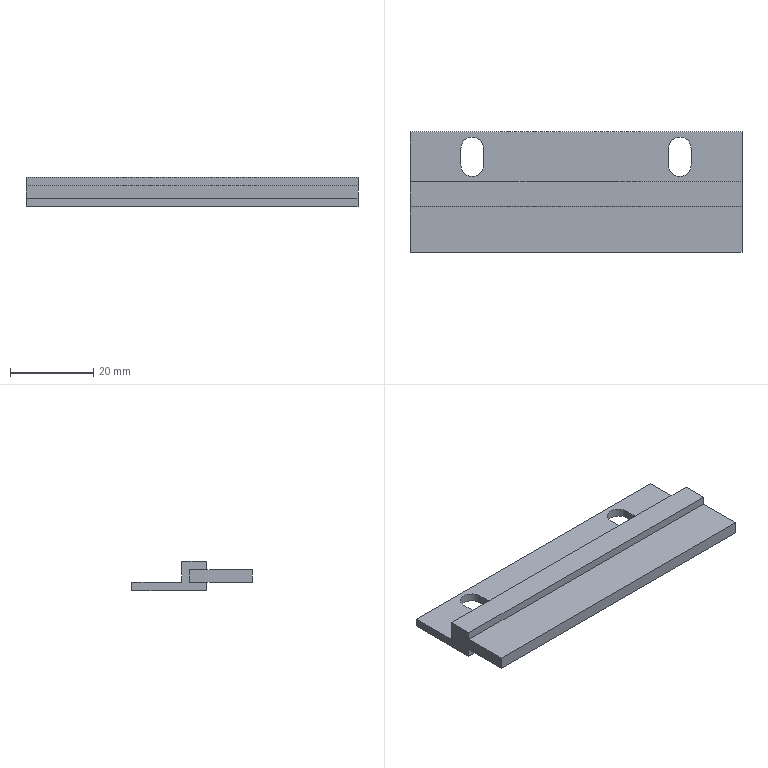Part | SolidWorks | features ICE 4, Extrusion 1, MirrorPattern 1 | 2 solids | 26 faces | box 80 x 29 x 7 mm | volume 7737 mm3 | plane 22 | cylinder 4 | commonest cylinder face diameters 5.5 x4
STEP:
#1=CARTESIAN_POINT('',(-40.,4.,5.));
#2=VERTEX_POINT('',#1);
#3=CARTESIAN_POINT('',(-40.,4.,2.));
#4=VERTEX_POINT('',#3);
#5=CARTESIAN_POINT('',(-40.,4.,5.));
#6=DIRECTION('',(0.,0.,-1.));
#7=VECTOR('',#6,1000.);
#8=LINE('',#5,#7);
#9=EDGE_CURVE('',#2,#4,#8,.T.);
#10=ORIENTED_EDGE('',*,*,#9,.T.);
#11=CARTESIAN_POINT('',(-40.,-11.,2.));
#12=VERTEX_POINT('',#11);
#13=CARTESIAN_POINT('',(-40.,-11.,2.));
#14=DIRECTION('',(0.,1.,0.));
#15=VECTOR('',#14,1000.);
#16=LINE('',#13,#15);
#17=EDGE_CURVE('',#12,#4,#16,.T.);
#18=ORIENTED_EDGE('',*,*,#17,.F.);
#19=CARTESIAN_POINT('',(-40.,-11.,5.));
#20=VERTEX_POINT('',#19);
#21=CARTESIAN_POINT('',(-40.,-11.,5.));
#22=DIRECTION('',(0.,0.,-1.));
#23=VECTOR('',#22,1000.);
#24=LINE('',#21,#23);
#25=EDGE_CURVE('',#20,#12,#24,.T.);
#26=ORIENTED_EDGE('',*,*,#25,.F.);
#27=CARTESIAN_POINT('',(-40.,-11.,5.));
#28=DIRECTION('',(0.,1.,0.));
#29=VECTOR('',#28,1000.);
#30=LINE('',#27,#29);
#31=EDGE_CURVE('',#20,#2,#30,.T.);
#32=ORIENTED_EDGE('',*,*,#31,.T.);
#33=EDGE_LOOP('',(#10,#18,#26,#32));
#34=FACE_OUTER_BOUND('',#33,.T.);
#35=CARTESIAN_POINT('',(-40.,-11.,5.));
#36=DIRECTION('',(1.,0.,0.));
#37=DIRECTION('',(0.,0.,-1.));
#38=AXIS2_PLACEMENT_3D('',#35,#36,#37);
#39=PLANE('',#38);
#40=ADVANCED_FACE('',(#34),#39,.F.);
#41=CARTESIAN_POINT('',(40.,4.,2.));
#42=VERTEX_POINT('',#41);
#43=CARTESIAN_POINT('',(-40.,4.,2.));
#44=DIRECTION('',(1.,0.,0.));
#45=VECTOR('',#44,1000.);
#46=LINE('',#43,#45);
#47=EDGE_CURVE('',#4,#42,#46,.T.);
#48=ORIENTED_EDGE('',*,*,#47,.T.);
#49=CARTESIAN_POINT('',(40.,-11.,2.));
#50=VERTEX_POINT('',#49);
#51=CARTESIAN_POINT('',(40.,-11.,2.));
#52=DIRECTION('',(0.,1.,0.));
#53=VECTOR('',#52,1000.);
#54=LINE('',#51,#53);
#55=EDGE_CURVE('',#50,#42,#54,.T.);
#56=ORIENTED_EDGE('',*,*,#55,.F.);
#57=CARTESIAN_POINT('',(-40.,-11.,2.));
#58=DIRECTION('',(1.,0.,0.));
#59=VECTOR('',#58,1000.);
#60=LINE('',#57,#59);
#61=EDGE_CURVE('',#12,#50,#60,.T.);
#62=ORIENTED_EDGE('',*,*,#61,.F.);
#63=ORIENTED_EDGE('',*,*,#17,.T.);
#64=EDGE_LOOP('',(#48,#56,#62,#63));
#65=FACE_OUTER_BOUND('',#64,.T.);
#66=CARTESIAN_POINT('',(-40.,-11.,2.));
#67=DIRECTION('',(0.,0.,1.));
#68=DIRECTION('',(1.,0.,0.));
#69=AXIS2_PLACEMENT_3D('',#66,#67,#68);
#70=PLANE('',#69);
#71=ADVANCED_FACE('',(#65),#70,.F.);
#72=CARTESIAN_POINT('',(40.,4.,5.));
#73=VERTEX_POINT('',#72);
#74=CARTESIAN_POINT('',(40.,4.,2.));
#75=DIRECTION('',(0.,0.,1.));
#76=VECTOR('',#75,1000.);
#77=LINE('',#74,#76);
#78=EDGE_CURVE('',#42,#73,#77,.T.);
#79=ORIENTED_EDGE('',*,*,#78,.T.);
#80=CARTESIAN_POINT('',(40.,-11.,5.));
#81=VERTEX_POINT('',#80);
#82=CARTESIAN_POINT('',(40.,-11.,5.));
#83=DIRECTION('',(0.,1.,0.));
#84=VECTOR('',#83,1000.);
#85=LINE('',#82,#84);
#86=EDGE_CURVE('',#81,#73,#85,.T.);
#87=ORIENTED_EDGE('',*,*,#86,.F.);
#88=CARTESIAN_POINT('',(40.,-11.,2.));
#89=DIRECTION('',(0.,0.,1.));
#90=VECTOR('',#89,1000.);
#91=LINE('',#88,#90);
#92=EDGE_CURVE('',#50,#81,#91,.T.);
#93=ORIENTED_EDGE('',*,*,#92,.F.);
#94=ORIENTED_EDGE('',*,*,#55,.T.);
#95=EDGE_LOOP('',(#79,#87,#93,#94));
#96=FACE_OUTER_BOUND('',#95,.T.);
#97=CARTESIAN_POINT('',(40.,-11.,2.));
#98=DIRECTION('',(-1.,0.,0.));
#99=DIRECTION('',(0.,0.,1.));
#100=AXIS2_PLACEMENT_3D('',#97,#98,#99);
#101=PLANE('',#100);
#102=ADVANCED_FACE('',(#96),#101,.F.);
#103=CARTESIAN_POINT('',(40.,4.,5.));
#104=DIRECTION('',(-1.,0.,0.));
#105=VECTOR('',#104,1000.);
#106=LINE('',#103,#105);
#107=EDGE_CURVE('',#73,#2,#106,.T.);
#108=ORIENTED_EDGE('',*,*,#107,.T.);
#109=ORIENTED_EDGE('',*,*,#31,.F.);
#110=CARTESIAN_POINT('',(40.,-11.,5.));
#111=DIRECTION('',(-1.,0.,0.));
#112=VECTOR('',#111,1000.);
#113=LINE('',#110,#112);
#114=EDGE_CURVE('',#81,#20,#113,.T.);
#115=ORIENTED_EDGE('',*,*,#114,.F.);
#116=ORIENTED_EDGE('',*,*,#86,.T.);
#117=EDGE_LOOP('',(#108,#109,#115,#116));
#118=FACE_OUTER_BOUND('',#117,.T.);
#119=CARTESIAN_POINT('',(40.,-11.,5.));
#120=DIRECTION('',(0.,0.,-1.));
#121=DIRECTION('',(-1.,0.,0.));
#122=AXIS2_PLACEMENT_3D('',#119,#120,#121);
#123=PLANE('',#122);
#124=ADVANCED_FACE('',(#118),#123,.F.);
#125=ORIENTED_EDGE('',*,*,#25,.T.);
#126=ORIENTED_EDGE('',*,*,#61,.T.);
#127=ORIENTED_EDGE('',*,*,#92,.T.);
#128=ORIENTED_EDGE('',*,*,#114,.T.);
#129=EDGE_LOOP('',(#125,#126,#127,#128));
#130=FACE_OUTER_BOUND('',#129,.T.);
#131=CARTESIAN_POINT('',(0.,-11.,0.));
#132=DIRECTION('',(0.,-1.,0.));
#133=DIRECTION('',(0.,0.,-1.));
#134=AXIS2_PLACEMENT_3D('',#131,#132,#133);
#135=PLANE('',#134);
#136=ADVANCED_FACE('',(#130),#135,.T.);
#137=ORIENTED_EDGE('',*,*,#9,.F.);
#138=ORIENTED_EDGE('',*,*,#107,.F.);
#139=ORIENTED_EDGE('',*,*,#78,.F.);
#140=ORIENTED_EDGE('',*,*,#47,.F.);
#141=EDGE_LOOP('',(#137,#138,#139,#140));
#142=FACE_OUTER_BOUND('',#141,.T.);
#143=CARTESIAN_POINT('',(0.,4.,0.));
#144=DIRECTION('',(0.,-1.,0.));
#145=DIRECTION('',(0.,0.,-1.));
#146=AXIS2_PLACEMENT_3D('',#143,#144,#145);
#147=PLANE('',#146);
#148=ADVANCED_FACE('',(#142),#147,.F.);
#149=CLOSED_SHELL('',(#40,#71,#102,#124,#136,#148));
#150=MANIFOLD_SOLID_BREP('',#149);
#151=CARTESIAN_POINT('',(40.,6.,2.));
#152=VERTEX_POINT('',#151);
#153=CARTESIAN_POINT('',(-40.,6.,2.));
#154=VERTEX_POINT('',#153);
#155=CARTESIAN_POINT('',(-40.,6.,2.));
#156=DIRECTION('',(-1.,0.,0.));
#157=VECTOR('',#156,1000.);
#158=LINE('',#155,#157);
#159=EDGE_CURVE('',#152,#154,#158,.T.);
#160=ORIENTED_EDGE('',*,*,#159,.F.);
#161=CARTESIAN_POINT('',(40.,18.,2.));
#162=VERTEX_POINT('',#161);
#163=CARTESIAN_POINT('',(40.,18.,2.));
#164=DIRECTION('',(0.,1.,0.));
#165=VECTOR('',#164,1000.);
#166=LINE('',#163,#165);
#167=EDGE_CURVE('',#152,#162,#166,.T.);
#168=ORIENTED_EDGE('',*,*,#167,.T.);
#169=CARTESIAN_POINT('',(-40.,18.,2.));
#170=VERTEX_POINT('',#169);
#171=CARTESIAN_POINT('',(-40.,18.,2.));
#172=DIRECTION('',(-1.,0.,0.));
#173=VECTOR('',#172,1000.);
#174=LINE('',#171,#173);
#175=EDGE_CURVE('',#162,#170,#174,.T.);
#176=ORIENTED_EDGE('',*,*,#175,.T.);
#177=CARTESIAN_POINT('',(-40.,18.,2.));
#178=DIRECTION('',(0.,-1.,0.));
#179=VECTOR('',#178,1000.);
#180=LINE('',#177,#179);
#181=EDGE_CURVE('',#170,#154,#180,.T.);
#182=ORIENTED_EDGE('',*,*,#181,.T.);
#183=EDGE_LOOP('',(#160,#168,#176,#182));
#184=FACE_OUTER_BOUND('',#183,.T.);
#185=CARTESIAN_POINT('',(-22.25,14.,2.));
#186=VERTEX_POINT('',#185);
#187=CARTESIAN_POINT('',(-27.75,14.,2.));
#188=VERTEX_POINT('',#187);
#189=CARTESIAN_POINT('',(-25.,14.,2.));
#190=DIRECTION('',(0.,0.,1.));
#191=DIRECTION('',(1.,0.,0.));
#192=AXIS2_PLACEMENT_3D('',#189,#190,#191);
#193=CIRCLE('',#192,2.75);
#194=EDGE_CURVE('',#186,#188,#193,.T.);
#195=ORIENTED_EDGE('',*,*,#194,.F.);
#196=CARTESIAN_POINT('',(-22.25,10.,2.));
#197=VERTEX_POINT('',#196);
#198=CARTESIAN_POINT('',(-22.25,14.,2.));
#199=DIRECTION('',(0.,1.,0.));
#200=VECTOR('',#199,1000.);
#201=LINE('',#198,#200);
#202=EDGE_CURVE('',#197,#186,#201,.T.);
#203=ORIENTED_EDGE('',*,*,#202,.F.);
#204=CARTESIAN_POINT('',(-27.75,10.,2.));
#205=VERTEX_POINT('',#204);
#206=CARTESIAN_POINT('',(-25.,10.,2.));
#207=DIRECTION('',(0.,0.,1.));
#208=DIRECTION('',(1.,0.,0.));
#209=AXIS2_PLACEMENT_3D('',#206,#207,#208);
#210=CIRCLE('',#209,2.75);
#211=EDGE_CURVE('',#205,#197,#210,.T.);
#212=ORIENTED_EDGE('',*,*,#211,.F.);
#213=CARTESIAN_POINT('',(-27.75,14.,2.));
#214=DIRECTION('',(0.,-1.,0.));
#215=VECTOR('',#214,1000.);
#216=LINE('',#213,#215);
#217=EDGE_CURVE('',#188,#205,#216,.T.);
#218=ORIENTED_EDGE('',*,*,#217,.F.);
#219=EDGE_LOOP('',(#195,#203,#212,#218));
#220=FACE_BOUND('',#219,.T.);
#221=CARTESIAN_POINT('',(22.25,10.,2.));
#222=VERTEX_POINT('',#221);
#223=CARTESIAN_POINT('',(22.25,14.,2.));
#224=VERTEX_POINT('',#223);
#225=CARTESIAN_POINT('',(22.25,14.,2.));
#226=DIRECTION('',(0.,1.,0.));
#227=VECTOR('',#226,1000.);
#228=LINE('',#225,#227);
#229=EDGE_CURVE('',#222,#224,#228,.T.);
#230=ORIENTED_EDGE('',*,*,#229,.T.);
#231=CARTESIAN_POINT('',(27.75,14.,2.));
#232=VERTEX_POINT('',#231);
#233=CARTESIAN_POINT('',(25.,14.,2.));
#234=DIRECTION('',(0.,0.,-1.));
#235=DIRECTION('',(-1.,0.,0.));
#236=AXIS2_PLACEMENT_3D('',#233,#234,#235);
#237=CIRCLE('',#236,2.75);
#238=EDGE_CURVE('',#224,#232,#237,.T.);
#239=ORIENTED_EDGE('',*,*,#238,.T.);
#240=CARTESIAN_POINT('',(27.75,10.,2.));
#241=VERTEX_POINT('',#240);
#242=CARTESIAN_POINT('',(27.75,14.,2.));
#243=DIRECTION('',(0.,-1.,0.));
#244=VECTOR('',#243,1000.);
#245=LINE('',#242,#244);
#246=EDGE_CURVE('',#232,#241,#245,.T.);
#247=ORIENTED_EDGE('',*,*,#246,.T.);
#248=CARTESIAN_POINT('',(25.,10.,2.));
#249=DIRECTION('',(0.,0.,-1.));
#250=DIRECTION('',(-1.,0.,0.));
#251=AXIS2_PLACEMENT_3D('',#248,#249,#250);
#252=CIRCLE('',#251,2.75);
#253=EDGE_CURVE('',#241,#222,#252,.T.);
#254=ORIENTED_EDGE('',*,*,#253,.T.);
#255=EDGE_LOOP('',(#230,#239,#247,#254));
#256=FACE_BOUND('',#255,.T.);
#257=CARTESIAN_POINT('',(0.,0.,2.));
#258=DIRECTION('',(0.,0.,1.));
#259=DIRECTION('',(1.,0.,0.));
#260=AXIS2_PLACEMENT_3D('',#257,#258,#259);
#261=PLANE('',#260);
#262=ADVANCED_FACE('',(#184,#220,#256),#261,.T.);
#263=CARTESIAN_POINT('',(-40.,18.,0.));
#264=VERTEX_POINT('',#263);
#265=CARTESIAN_POINT('',(-40.,0.,0.));
#266=VERTEX_POINT('',#265);
#267=CARTESIAN_POINT('',(-40.,18.,0.));
#268=DIRECTION('',(0.,-1.,0.));
#269=VECTOR('',#268,1000.);
#270=LINE('',#267,#269);
#271=EDGE_CURVE('',#264,#266,#270,.T.);
#272=ORIENTED_EDGE('',*,*,#271,.F.);
#273=CARTESIAN_POINT('',(40.,18.,0.));
#274=VERTEX_POINT('',#273);
#275=CARTESIAN_POINT('',(-40.,18.,0.));
#276=DIRECTION('',(-1.,0.,0.));
#277=VECTOR('',#276,1000.);
#278=LINE('',#275,#277);
#279=EDGE_CURVE('',#274,#264,#278,.T.);
#280=ORIENTED_EDGE('',*,*,#279,.F.);
#281=CARTESIAN_POINT('',(40.,0.,0.));
#282=VERTEX_POINT('',#281);
#283=CARTESIAN_POINT('',(40.,18.,0.));
#284=DIRECTION('',(0.,1.,0.));
#285=VECTOR('',#284,1000.);
#286=LINE('',#283,#285);
#287=EDGE_CURVE('',#282,#274,#286,.T.);
#288=ORIENTED_EDGE('',*,*,#287,.F.);
#289=CARTESIAN_POINT('',(-40.,0.,0.));
#290=DIRECTION('',(1.,0.,0.));
#291=VECTOR('',#290,1000.);
#292=LINE('',#289,#291);
#293=EDGE_CURVE('',#266,#282,#292,.T.);
#294=ORIENTED_EDGE('',*,*,#293,.F.);
#295=EDGE_LOOP('',(#272,#280,#288,#294));
#296=FACE_OUTER_BOUND('',#295,.T.);
#297=CARTESIAN_POINT('',(-22.25,10.,0.));
#298=VERTEX_POINT('',#297);
#299=CARTESIAN_POINT('',(-22.25,14.,0.));
#300=VERTEX_POINT('',#299);
#301=CARTESIAN_POINT('',(-22.25,0.,0.));
#302=DIRECTION('',(0.,1.,0.));
#303=VECTOR('',#302,1000.);
#304=LINE('',#301,#303);
#305=EDGE_CURVE('',#298,#300,#304,.T.);
#306=ORIENTED_EDGE('',*,*,#305,.T.);
#307=CARTESIAN_POINT('',(-27.75,14.,0.));
#308=VERTEX_POINT('',#307);
#309=CARTESIAN_POINT('',(-25.,14.,0.));
#310=DIRECTION('',(0.,0.,1.));
#311=DIRECTION('',(1.,0.,0.));
#312=AXIS2_PLACEMENT_3D('',#309,#310,#311);
#313=CIRCLE('',#312,2.75);
#314=EDGE_CURVE('',#300,#308,#313,.T.);
#315=ORIENTED_EDGE('',*,*,#314,.T.);
#316=CARTESIAN_POINT('',(-27.75,10.,0.));
#317=VERTEX_POINT('',#316);
#318=CARTESIAN_POINT('',(-27.75,0.,0.));
#319=DIRECTION('',(0.,-1.,0.));
#320=VECTOR('',#319,1000.);
#321=LINE('',#318,#320);
#322=EDGE_CURVE('',#308,#317,#321,.T.);
#323=ORIENTED_EDGE('',*,*,#322,.T.);
#324=CARTESIAN_POINT('',(-25.,10.,0.));
#325=DIRECTION('',(0.,0.,1.));
#326=DIRECTION('',(1.,0.,0.));
#327=AXIS2_PLACEMENT_3D('',#324,#325,#326);
#328=CIRCLE('',#327,2.75);
#329=EDGE_CURVE('',#317,#298,#328,.T.);
#330=ORIENTED_EDGE('',*,*,#329,.T.);
#331=EDGE_LOOP('',(#306,#315,#323,#330));
#332=FACE_BOUND('',#331,.T.);
#333=CARTESIAN_POINT('',(22.25,14.,0.));
#334=VERTEX_POINT('',#333);
#335=CARTESIAN_POINT('',(27.75,14.,0.));
#336=VERTEX_POINT('',#335);
#337=CARTESIAN_POINT('',(25.,14.,0.));
#338=DIRECTION('',(0.,0.,-1.));
#339=DIRECTION('',(1.,0.,0.));
#340=AXIS2_PLACEMENT_3D('',#337,#338,#339);
#341=CIRCLE('',#340,2.75);
#342=EDGE_CURVE('',#334,#336,#341,.T.);
#343=ORIENTED_EDGE('',*,*,#342,.F.);
#344=CARTESIAN_POINT('',(22.25,10.,0.));
#345=VERTEX_POINT('',#344);
#346=CARTESIAN_POINT('',(22.25,0.,0.));
#347=DIRECTION('',(0.,1.,0.));
#348=VECTOR('',#347,1000.);
#349=LINE('',#346,#348);
#350=EDGE_CURVE('',#345,#334,#349,.T.);
#351=ORIENTED_EDGE('',*,*,#350,.F.);
#352=CARTESIAN_POINT('',(27.75,10.,0.));
#353=VERTEX_POINT('',#352);
#354=CARTESIAN_POINT('',(25.,10.,0.));
#355=DIRECTION('',(0.,0.,-1.));
#356=DIRECTION('',(1.,0.,0.));
#357=AXIS2_PLACEMENT_3D('',#354,#355,#356);
#358=CIRCLE('',#357,2.75);
#359=EDGE_CURVE('',#353,#345,#358,.T.);
#360=ORIENTED_EDGE('',*,*,#359,.F.);
#361=CARTESIAN_POINT('',(27.75,0.,0.));
#362=DIRECTION('',(0.,-1.,0.));
#363=VECTOR('',#362,1000.);
#364=LINE('',#361,#363);
#365=EDGE_CURVE('',#336,#353,#364,.T.);
#366=ORIENTED_EDGE('',*,*,#365,.F.);
#367=EDGE_LOOP('',(#343,#351,#360,#366));
#368=FACE_BOUND('',#367,.T.);
#369=CARTESIAN_POINT('',(0.,0.,0.));
#370=DIRECTION('',(0.,0.,1.));
#371=DIRECTION('',(1.,0.,0.));
#372=AXIS2_PLACEMENT_3D('',#369,#370,#371);
#373=PLANE('',#372);
#374=ADVANCED_FACE('',(#296,#332,#368),#373,.F.);
#375=ORIENTED_EDGE('',*,*,#271,.T.);
#376=CARTESIAN_POINT('',(-40.,0.,2.));
#377=VERTEX_POINT('',#376);
#378=CARTESIAN_POINT('',(-40.,0.,2.));
#379=DIRECTION('',(0.,0.,-1.));
#380=VECTOR('',#379,1000.);
#381=LINE('',#378,#380);
#382=EDGE_CURVE('',#377,#266,#381,.T.);
#383=ORIENTED_EDGE('',*,*,#382,.F.);
#384=CARTESIAN_POINT('',(-40.,4.,2.));
#385=VERTEX_POINT('',#384);
#386=CARTESIAN_POINT('',(-40.,18.,2.));
#387=DIRECTION('',(0.,-1.,0.));
#388=VECTOR('',#387,1000.);
#389=LINE('',#386,#388);
#390=EDGE_CURVE('',#385,#377,#389,.T.);
#391=ORIENTED_EDGE('',*,*,#390,.F.);
#392=CARTESIAN_POINT('',(-40.,4.,5.));
#393=VERTEX_POINT('',#392);
#394=CARTESIAN_POINT('',(-40.,4.,5.));
#395=DIRECTION('',(0.,0.,-1.));
#396=VECTOR('',#395,1000.);
#397=LINE('',#394,#396);
#398=EDGE_CURVE('',#393,#385,#397,.T.);
#399=ORIENTED_EDGE('',*,*,#398,.F.);
#400=CARTESIAN_POINT('',(-40.,0.,5.));
#401=VERTEX_POINT('',#400);
#402=CARTESIAN_POINT('',(-40.,-80.025,5.));
#403=DIRECTION('',(0.,1.,0.));
#404=VECTOR('',#403,1000.);
#405=LINE('',#402,#404);
#406=EDGE_CURVE('',#401,#393,#405,.T.);
#407=ORIENTED_EDGE('',*,*,#406,.F.);
#408=CARTESIAN_POINT('',(-40.,0.,7.));
#409=VERTEX_POINT('',#408);
#410=CARTESIAN_POINT('',(-40.,0.,5.));
#411=DIRECTION('',(0.,0.,-1.));
#412=VECTOR('',#411,1000.);
#413=LINE('',#410,#412);
#414=EDGE_CURVE('',#409,#401,#413,.T.);
#415=ORIENTED_EDGE('',*,*,#414,.F.);
#416=CARTESIAN_POINT('',(-40.,6.,7.));
#417=VERTEX_POINT('',#416);
#418=CARTESIAN_POINT('',(-40.,-80.025,7.));
#419=DIRECTION('',(0.,1.,0.));
#420=VECTOR('',#419,1000.);
#421=LINE('',#418,#420);
#422=EDGE_CURVE('',#409,#417,#421,.T.);
#423=ORIENTED_EDGE('',*,*,#422,.T.);
#424=CARTESIAN_POINT('',(-40.,6.,5.));
#425=DIRECTION('',(0.,0.,-1.));
#426=VECTOR('',#425,1000.);
#427=LINE('',#424,#426);
#428=EDGE_CURVE('',#417,#154,#427,.T.);
#429=ORIENTED_EDGE('',*,*,#428,.T.);
#430=ORIENTED_EDGE('',*,*,#181,.F.);
#431=CARTESIAN_POINT('',(-40.,18.,2.));
#432=DIRECTION('',(0.,0.,-1.));
#433=VECTOR('',#432,1000.);
#434=LINE('',#431,#433);
#435=EDGE_CURVE('',#170,#264,#434,.T.);
#436=ORIENTED_EDGE('',*,*,#435,.T.);
#437=EDGE_LOOP('',(#375,#383,#391,#399,#407,#415,#423,#429,#430,#436));
#438=FACE_OUTER_BOUND('',#437,.T.);
#439=CARTESIAN_POINT('',(-40.,18.,2.));
#440=DIRECTION('',(1.,0.,0.));
#441=DIRECTION('',(0.,1.,0.));
#442=AXIS2_PLACEMENT_3D('',#439,#440,#441);
#443=PLANE('',#442);
#444=ADVANCED_FACE('',(#438),#443,.F.);
#445=ORIENTED_EDGE('',*,*,#293,.T.);
#446=CARTESIAN_POINT('',(40.,0.,2.));
#447=VERTEX_POINT('',#446);
#448=CARTESIAN_POINT('',(40.,0.,2.));
#449=DIRECTION('',(0.,0.,-1.));
#450=VECTOR('',#449,1000.);
#451=LINE('',#448,#450);
#452=EDGE_CURVE('',#447,#282,#451,.T.);
#453=ORIENTED_EDGE('',*,*,#452,.F.);
#454=CARTESIAN_POINT('',(-40.,0.,2.));
#455=DIRECTION('',(1.,0.,0.));
#456=VECTOR('',#455,1000.);
#457=LINE('',#454,#456);
#458=EDGE_CURVE('',#377,#447,#457,.T.);
#459=ORIENTED_EDGE('',*,*,#458,.F.);
#460=ORIENTED_EDGE('',*,*,#382,.T.);
#461=EDGE_LOOP('',(#445,#453,#459,#460));
#462=FACE_OUTER_BOUND('',#461,.T.);
#463=CARTESIAN_POINT('',(-40.,0.,2.));
#464=DIRECTION('',(0.,1.,0.));
#465=DIRECTION('',(0.,0.,1.));
#466=AXIS2_PLACEMENT_3D('',#463,#464,#465);
#467=PLANE('',#466);
#468=ADVANCED_FACE('',(#462),#467,.F.);
#469=ORIENTED_EDGE('',*,*,#287,.T.);
#470=CARTESIAN_POINT('',(40.,18.,2.));
#471=DIRECTION('',(0.,0.,-1.));
#472=VECTOR('',#471,1000.);
#473=LINE('',#470,#472);
#474=EDGE_CURVE('',#162,#274,#473,.T.);
#475=ORIENTED_EDGE('',*,*,#474,.F.);
#476=ORIENTED_EDGE('',*,*,#167,.F.);
#477=CARTESIAN_POINT('',(40.,6.,7.));
#478=VERTEX_POINT('',#477);
#479=CARTESIAN_POINT('',(40.,6.,5.));
#480=DIRECTION('',(0.,0.,-1.));
#481=VECTOR('',#480,1000.);
#482=LINE('',#479,#481);
#483=EDGE_CURVE('',#478,#152,#482,.T.);
#484=ORIENTED_EDGE('',*,*,#483,.F.);
#485=CARTESIAN_POINT('',(40.,0.,7.));
#486=VERTEX_POINT('',#485);
#487=CARTESIAN_POINT('',(40.,-80.025,7.));
#488=DIRECTION('',(0.,1.,0.));
#489=VECTOR('',#488,1000.);
#490=LINE('',#487,#489);
#491=EDGE_CURVE('',#486,#478,#490,.T.);
#492=ORIENTED_EDGE('',*,*,#491,.F.);
#493=CARTESIAN_POINT('',(40.,0.,5.));
#494=VERTEX_POINT('',#493);
#495=CARTESIAN_POINT('',(40.,0.,5.));
#496=DIRECTION('',(0.,0.,1.));
#497=VECTOR('',#496,1000.);
#498=LINE('',#495,#497);
#499=EDGE_CURVE('',#494,#486,#498,.T.);
#500=ORIENTED_EDGE('',*,*,#499,.F.);
#501=CARTESIAN_POINT('',(40.,4.,5.));
#502=VERTEX_POINT('',#501);
#503=CARTESIAN_POINT('',(40.,-80.025,5.));
#504=DIRECTION('',(0.,1.,0.));
#505=VECTOR('',#504,1000.);
#506=LINE('',#503,#505);
#507=EDGE_CURVE('',#494,#502,#506,.T.);
#508=ORIENTED_EDGE('',*,*,#507,.T.);
#509=CARTESIAN_POINT('',(40.,4.,2.));
#510=VERTEX_POINT('',#509);
#511=CARTESIAN_POINT('',(40.,4.,5.));
#512=DIRECTION('',(0.,0.,-1.));
#513=VECTOR('',#512,1000.);
#514=LINE('',#511,#513);
#515=EDGE_CURVE('',#502,#510,#514,.T.);
#516=ORIENTED_EDGE('',*,*,#515,.T.);
#517=CARTESIAN_POINT('',(40.,18.,2.));
#518=DIRECTION('',(0.,1.,0.));
#519=VECTOR('',#518,1000.);
#520=LINE('',#517,#519);
#521=EDGE_CURVE('',#447,#510,#520,.T.);
#522=ORIENTED_EDGE('',*,*,#521,.F.);
#523=ORIENTED_EDGE('',*,*,#452,.T.);
#524=EDGE_LOOP('',(#469,#475,#476,#484,#492,#500,#508,#516,#522,#523));
#525=FACE_OUTER_BOUND('',#524,.T.);
#526=CARTESIAN_POINT('',(40.,18.,2.));
#527=DIRECTION('',(-1.,0.,0.));
#528=DIRECTION('',(0.,0.,1.));
#529=AXIS2_PLACEMENT_3D('',#526,#527,#528);
#530=PLANE('',#529);
#531=ADVANCED_FACE('',(#525),#530,.F.);
#532=ORIENTED_EDGE('',*,*,#279,.T.);
#533=ORIENTED_EDGE('',*,*,#435,.F.);
#534=ORIENTED_EDGE('',*,*,#175,.F.);
#535=ORIENTED_EDGE('',*,*,#474,.T.);
#536=EDGE_LOOP('',(#532,#533,#534,#535));
#537=FACE_OUTER_BOUND('',#536,.T.);
#538=CARTESIAN_POINT('',(-40.,18.,2.));
#539=DIRECTION('',(0.,-1.,0.));
#540=DIRECTION('',(1.,0.,0.));
#541=AXIS2_PLACEMENT_3D('',#538,#539,#540);
#542=PLANE('',#541);
#543=ADVANCED_FACE('',(#537),#542,.F.);
#544=CARTESIAN_POINT('',(-40.,4.,2.));
#545=DIRECTION('',(1.,0.,0.));
#546=VECTOR('',#545,1000.);
#547=LINE('',#544,#546);
#548=EDGE_CURVE('',#385,#510,#547,.T.);
#549=ORIENTED_EDGE('',*,*,#548,.F.);
#550=ORIENTED_EDGE('',*,*,#390,.T.);
#551=ORIENTED_EDGE('',*,*,#458,.T.);
#552=ORIENTED_EDGE('',*,*,#521,.T.);
#553=EDGE_LOOP('',(#549,#550,#551,#552));
#554=FACE_OUTER_BOUND('',#553,.T.);
#555=CARTESIAN_POINT('',(0.,0.,2.));
#556=DIRECTION('',(0.,0.,1.));
#557=DIRECTION('',(1.,0.,0.));
#558=AXIS2_PLACEMENT_3D('',#555,#556,#557);
#559=PLANE('',#558);
#560=ADVANCED_FACE('',(#554),#559,.T.);
#561=ORIENTED_EDGE('',*,*,#548,.T.);
#562=ORIENTED_EDGE('',*,*,#515,.F.);
#563=CARTESIAN_POINT('',(-40.,4.,5.));
#564=DIRECTION('',(1.,0.,0.));
#565=VECTOR('',#564,1000.);
#566=LINE('',#563,#565);
#567=EDGE_CURVE('',#393,#502,#566,.T.);
#568=ORIENTED_EDGE('',*,*,#567,.F.);
#569=ORIENTED_EDGE('',*,*,#398,.T.);
#570=EDGE_LOOP('',(#561,#562,#568,#569));
#571=FACE_OUTER_BOUND('',#570,.T.);
#572=CARTESIAN_POINT('',(-40.,4.,5.));
#573=DIRECTION('',(0.,1.,0.));
#574=DIRECTION('',(0.,0.,1.));
#575=AXIS2_PLACEMENT_3D('',#572,#573,#574);
#576=PLANE('',#575);
#577=ADVANCED_FACE('',(#571),#576,.F.);
#578=ORIENTED_EDGE('',*,*,#159,.T.);
#579=ORIENTED_EDGE('',*,*,#428,.F.);
#580=CARTESIAN_POINT('',(-40.,6.,7.));
#581=DIRECTION('',(1.,0.,0.));
#582=VECTOR('',#581,1000.);
#583=LINE('',#580,#582);
#584=EDGE_CURVE('',#417,#478,#583,.T.);
#585=ORIENTED_EDGE('',*,*,#584,.T.);
#586=ORIENTED_EDGE('',*,*,#483,.T.);
#587=EDGE_LOOP('',(#578,#579,#585,#586));
#588=FACE_OUTER_BOUND('',#587,.T.);
#589=CARTESIAN_POINT('',(-40.,6.,5.));
#590=DIRECTION('',(0.,-1.,0.));
#591=DIRECTION('',(1.,0.,0.));
#592=AXIS2_PLACEMENT_3D('',#589,#590,#591);
#593=PLANE('',#592);
#594=ADVANCED_FACE('',(#588),#593,.F.);
#595=ORIENTED_EDGE('',*,*,#406,.T.);
#596=ORIENTED_EDGE('',*,*,#567,.T.);
#597=ORIENTED_EDGE('',*,*,#507,.F.);
#598=CARTESIAN_POINT('',(-40.,0.,5.));
#599=DIRECTION('',(1.,0.,0.));
#600=VECTOR('',#599,1000.);
#601=LINE('',#598,#600);
#602=EDGE_CURVE('',#401,#494,#601,.T.);
#603=ORIENTED_EDGE('',*,*,#602,.F.);
#604=EDGE_LOOP('',(#595,#596,#597,#603));
#605=FACE_OUTER_BOUND('',#604,.T.);
#606=CARTESIAN_POINT('',(-40.,-80.025,5.));
#607=DIRECTION('',(0.,0.,-1.));
#608=DIRECTION('',(-1.,0.,0.));
#609=AXIS2_PLACEMENT_3D('',#606,#607,#608);
#610=PLANE('',#609);
#611=ADVANCED_FACE('',(#605),#610,.T.);
#612=CARTESIAN_POINT('',(-40.,0.,7.));
#613=DIRECTION('',(-1.,0.,0.));
#614=VECTOR('',#613,1000.);
#615=LINE('',#612,#614);
#616=EDGE_CURVE('',#486,#409,#615,.T.);
#617=ORIENTED_EDGE('',*,*,#616,.F.);
#618=ORIENTED_EDGE('',*,*,#491,.T.);
#619=ORIENTED_EDGE('',*,*,#584,.F.);
#620=ORIENTED_EDGE('',*,*,#422,.F.);
#621=EDGE_LOOP('',(#617,#618,#619,#620));
#622=FACE_OUTER_BOUND('',#621,.T.);
#623=CARTESIAN_POINT('',(-40.,-80.025,7.));
#624=DIRECTION('',(0.,0.,1.));
#625=DIRECTION('',(1.,0.,0.));
#626=AXIS2_PLACEMENT_3D('',#623,#624,#625);
#627=PLANE('',#626);
#628=ADVANCED_FACE('',(#622),#627,.T.);
#629=ORIENTED_EDGE('',*,*,#414,.T.);
#630=ORIENTED_EDGE('',*,*,#602,.T.);
#631=ORIENTED_EDGE('',*,*,#499,.T.);
#632=ORIENTED_EDGE('',*,*,#616,.T.);
#633=EDGE_LOOP('',(#629,#630,#631,#632));
#634=FACE_OUTER_BOUND('',#633,.T.);
#635=CARTESIAN_POINT('',(-40.,0.,2.));
#636=DIRECTION('',(0.,1.,0.));
#637=DIRECTION('',(0.,0.,1.));
#638=AXIS2_PLACEMENT_3D('',#635,#636,#637);
#639=PLANE('',#638);
#640=ADVANCED_FACE('',(#634),#639,.F.);
#641=CARTESIAN_POINT('',(-22.25,14.,-3.));
#642=DIRECTION('',(0.,0.,1.));
#643=VECTOR('',#642,1000.);
#644=LINE('',#641,#643);
#645=EDGE_CURVE('',#300,#186,#644,.T.);
#646=ORIENTED_EDGE('',*,*,#645,.T.);
#647=ORIENTED_EDGE('',*,*,#194,.T.);
#648=CARTESIAN_POINT('',(-27.75,14.,-3.));
#649=DIRECTION('',(0.,0.,1.));
#650=VECTOR('',#649,1000.);
#651=LINE('',#648,#650);
#652=EDGE_CURVE('',#308,#188,#651,.T.);
#653=ORIENTED_EDGE('',*,*,#652,.F.);
#654=ORIENTED_EDGE('',*,*,#314,.F.);
#655=EDGE_LOOP('',(#646,#647,#653,#654));
#656=FACE_OUTER_BOUND('',#655,.T.);
#657=CARTESIAN_POINT('',(-25.,14.,-3.));
#658=DIRECTION('',(0.,0.,1.));
#659=DIRECTION('',(1.,0.,0.));
#660=AXIS2_PLACEMENT_3D('',#657,#658,#659);
#661=CYLINDRICAL_SURFACE('',#660,2.75);
#662=ADVANCED_FACE('',(#656),#661,.F.);
#663=CARTESIAN_POINT('',(-22.25,10.,-3.));
#664=DIRECTION('',(0.,0.,1.));
#665=VECTOR('',#664,1000.);
#666=LINE('',#663,#665);
#667=EDGE_CURVE('',#298,#197,#666,.T.);
#668=ORIENTED_EDGE('',*,*,#667,.T.);
#669=ORIENTED_EDGE('',*,*,#202,.T.);
#670=ORIENTED_EDGE('',*,*,#645,.F.);
#671=ORIENTED_EDGE('',*,*,#305,.F.);
#672=EDGE_LOOP('',(#668,#669,#670,#671));
#673=FACE_OUTER_BOUND('',#672,.T.);
#674=CARTESIAN_POINT('',(-22.25,14.,-3.));
#675=DIRECTION('',(1.,0.,0.));
#676=DIRECTION('',(0.,1.,0.));
#677=AXIS2_PLACEMENT_3D('',#674,#675,#676);
#678=PLANE('',#677);
#679=ADVANCED_FACE('',(#673),#678,.F.);
#680=CARTESIAN_POINT('',(-27.75,10.,-3.));
#681=DIRECTION('',(0.,0.,1.));
#682=VECTOR('',#681,1000.);
#683=LINE('',#680,#682);
#684=EDGE_CURVE('',#317,#205,#683,.T.);
#685=ORIENTED_EDGE('',*,*,#684,.T.);
#686=ORIENTED_EDGE('',*,*,#211,.T.);
#687=ORIENTED_EDGE('',*,*,#667,.F.);
#688=ORIENTED_EDGE('',*,*,#329,.F.);
#689=EDGE_LOOP('',(#685,#686,#687,#688));
#690=FACE_OUTER_BOUND('',#689,.T.);
#691=CARTESIAN_POINT('',(-25.,10.,-3.));
#692=DIRECTION('',(0.,0.,1.));
#693=DIRECTION('',(1.,0.,0.));
#694=AXIS2_PLACEMENT_3D('',#691,#692,#693);
#695=CYLINDRICAL_SURFACE('',#694,2.75);
#696=ADVANCED_FACE('',(#690),#695,.F.);
#697=ORIENTED_EDGE('',*,*,#652,.T.);
#698=ORIENTED_EDGE('',*,*,#217,.T.);
#699=ORIENTED_EDGE('',*,*,#684,.F.);
#700=ORIENTED_EDGE('',*,*,#322,.F.);
#701=EDGE_LOOP('',(#697,#698,#699,#700));
#702=FACE_OUTER_BOUND('',#701,.T.);
#703=CARTESIAN_POINT('',(-27.75,14.,-3.));
#704=DIRECTION('',(-1.,0.,0.));
#705=DIRECTION('',(0.,-1.,0.));
#706=AXIS2_PLACEMENT_3D('',#703,#704,#705);
#707=PLANE('',#706);
#708=ADVANCED_FACE('',(#702),#707,.F.);
#709=ORIENTED_EDGE('',*,*,#342,.T.);
#710=CARTESIAN_POINT('',(27.75,14.,-3.));
#711=DIRECTION('',(0.,0.,1.));
#712=VECTOR('',#711,1000.);
#713=LINE('',#710,#712);
#714=EDGE_CURVE('',#336,#232,#713,.T.);
#715=ORIENTED_EDGE('',*,*,#714,.T.);
#716=ORIENTED_EDGE('',*,*,#238,.F.);
#717=CARTESIAN_POINT('',(22.25,14.,-3.));
#718=DIRECTION('',(0.,0.,1.));
#719=VECTOR('',#718,1000.);
#720=LINE('',#717,#719);
#721=EDGE_CURVE('',#334,#224,#720,.T.);
#722=ORIENTED_EDGE('',*,*,#721,.F.);
#723=EDGE_LOOP('',(#709,#715,#716,#722));
#724=FACE_OUTER_BOUND('',#723,.T.);
#725=CARTESIAN_POINT('',(25.,14.,-3.));
#726=DIRECTION('',(0.,0.,1.));
#727=DIRECTION('',(1.,0.,0.));
#728=AXIS2_PLACEMENT_3D('',#725,#726,#727);
#729=CYLINDRICAL_SURFACE('',#728,2.75);
#730=ADVANCED_FACE('',(#724),#729,.F.);
#731=ORIENTED_EDGE('',*,*,#365,.T.);
#732=CARTESIAN_POINT('',(27.75,10.,-3.));
#733=DIRECTION('',(0.,0.,1.));
#734=VECTOR('',#733,1000.);
#735=LINE('',#732,#734);
#736=EDGE_CURVE('',#353,#241,#735,.T.);
#737=ORIENTED_EDGE('',*,*,#736,.T.);
#738=ORIENTED_EDGE('',*,*,#246,.F.);
#739=ORIENTED_EDGE('',*,*,#714,.F.);
#740=EDGE_LOOP('',(#731,#737,#738,#739));
#741=FACE_OUTER_BOUND('',#740,.T.);
#742=CARTESIAN_POINT('',(27.75,14.,-3.));
#743=DIRECTION('',(-1.,0.,0.));
#744=DIRECTION('',(0.,-1.,0.));
#745=AXIS2_PLACEMENT_3D('',#742,#743,#744);
#746=PLANE('',#745);
#747=ADVANCED_FACE('',(#741),#746,.T.);
#748=ORIENTED_EDGE('',*,*,#359,.T.);
#749=CARTESIAN_POINT('',(22.25,10.,-3.));
#750=DIRECTION('',(0.,0.,1.));
#751=VECTOR('',#750,1000.);
#752=LINE('',#749,#751);
#753=EDGE_CURVE('',#345,#222,#752,.T.);
#754=ORIENTED_EDGE('',*,*,#753,.T.);
#755=ORIENTED_EDGE('',*,*,#253,.F.);
#756=ORIENTED_EDGE('',*,*,#736,.F.);
#757=EDGE_LOOP('',(#748,#754,#755,#756));
#758=FACE_OUTER_BOUND('',#757,.T.);
#759=CARTESIAN_POINT('',(25.,10.,-3.));
#760=DIRECTION('',(0.,0.,1.));
#761=DIRECTION('',(1.,0.,0.));
#762=AXIS2_PLACEMENT_3D('',#759,#760,#761);
#763=CYLINDRICAL_SURFACE('',#762,2.75);
#764=ADVANCED_FACE('',(#758),#763,.F.);
#765=ORIENTED_EDGE('',*,*,#350,.T.);
#766=ORIENTED_EDGE('',*,*,#721,.T.);
#767=ORIENTED_EDGE('',*,*,#229,.F.);
#768=ORIENTED_EDGE('',*,*,#753,.F.);
#769=EDGE_LOOP('',(#765,#766,#767,#768));
#770=FACE_OUTER_BOUND('',#769,.T.);
#771=CARTESIAN_POINT('',(22.25,14.,-3.));
#772=DIRECTION('',(1.,0.,0.));
#773=DIRECTION('',(0.,1.,0.));
#774=AXIS2_PLACEMENT_3D('',#771,#772,#773);
#775=PLANE('',#774);
#776=ADVANCED_FACE('',(#770),#775,.T.);
#777=CLOSED_SHELL('',(#262,#374,#444,#468,#531,#543,#560,#577,#594,#611,#628,#640,#662,#679,#696,#708,#730,#747,#764,#776));
#778=MANIFOLD_SOLID_BREP('',#777);
#779=CARTESIAN_POINT('',(0.,0.,0.));
#780=DIRECTION('',(0.,0.,1.));
#781=DIRECTION('',(1.,0.,0.));
#782=AXIS2_PLACEMENT_3D('',#779,#780,#781);
#783=(LENGTH_UNIT()NAMED_UNIT(*)SI_UNIT(.MILLI.,.METRE.));
#784=UNCERTAINTY_MEASURE_WITH_UNIT(LENGTH_MEASURE(0.00001),#783,'','');
#785=(NAMED_UNIT(*)PLANE_ANGLE_UNIT()SI_UNIT($,.RADIAN.));
#786=(NAMED_UNIT(*)SI_UNIT($,.STERADIAN.)SOLID_ANGLE_UNIT());
#787=(GEOMETRIC_REPRESENTATION_CONTEXT(3)GLOBAL_UNCERTAINTY_ASSIGNED_CONTEXT((#784))GLOBAL_UNIT_ASSIGNED_CONTEXT((#783,#785,#786))REPRESENTATION_CONTEXT('',''));
#788=ADVANCED_BREP_SHAPE_REPRESENTATION('',(#150,#778,#782),#787);